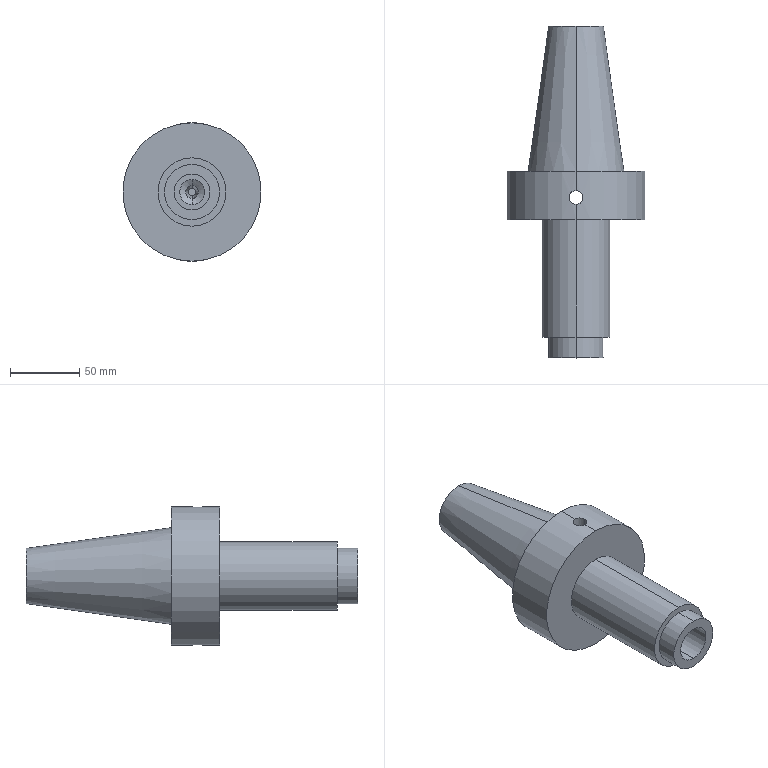Part | SolidWorks | features ICE 2, 3DProfileFeature 1, HoleWzd 1, RevolutionThin 1 | 1 solid | 31 faces | box 100 x 240 x 100 mm | volume 634336 mm3 | cylinder 16 | plane 9 | cone 6 | commonest cylinder face diameters 9.4 x4 10 x2 18 x2 26 x2 40 x2 49.4 x2
STEP:
#1=CARTESIAN_POINT('',(0.,220.,2.654));
#2=VERTEX_POINT('',#1);
#3=CARTESIAN_POINT('',(0.,220.,-2.654));
#4=VERTEX_POINT('',#3);
#5=CARTESIAN_POINT('',(0.,220.,0.));
#6=DIRECTION('',(0.,-1.,0.));
#7=DIRECTION('',(0.,0.,-1.));
#8=AXIS2_PLACEMENT_3D('',#5,#6,#7);
#9=CIRCLE('',#8,2.654);
#10=EDGE_CURVE('',#2,#4,#9,.T.);
#11=ORIENTED_EDGE('',*,*,#10,.F.);
#12=CARTESIAN_POINT('',(0.,121.,16.797));
#13=VERTEX_POINT('',#12);
#14=CARTESIAN_POINT('',(0.,220.,2.654));
#15=DIRECTION('',(0.,-0.9899,0.1414));
#16=VECTOR('',#15,1000.);
#17=LINE('',#14,#16);
#18=EDGE_CURVE('',#2,#13,#17,.T.);
#19=ORIENTED_EDGE('',*,*,#18,.T.);
#20=CARTESIAN_POINT('',(-3.,120.,16.672));
#21=VERTEX_POINT('',#20);
#22=CARTESIAN_POINT('',(-3.,120.,16.672));
#23=CARTESIAN_POINT('',(-2.567,120.325,16.703));
#24=CARTESIAN_POINT('',(-2.094,120.572,16.735));
#25=CARTESIAN_POINT('',(-1.326,120.829,16.771));
#26=CARTESIAN_POINT('',(-1.064,120.893,16.781));
#27=CARTESIAN_POINT('',(-0.5365,120.978,16.794));
#28=CARTESIAN_POINT('',(-0.2698,121.,16.797));
#29=CARTESIAN_POINT('',(0.,121.,16.797));
#30=B_SPLINE_CURVE_WITH_KNOTS('',3,(#22,#23,#24,#25,#26,#27,#28,#29),.UNSPECIFIED.,.F.,.F.,(4,2,2,4),(0.000000329,0.001604,0.002405,0.003207),.UNSPECIFIED.);
#31=EDGE_CURVE('',#21,#13,#30,.T.);
#32=ORIENTED_EDGE('',*,*,#31,.F.);
#33=CARTESIAN_POINT('',(-3.,120.,-16.672));
#34=VERTEX_POINT('',#33);
#35=CARTESIAN_POINT('',(0.,120.,0.));
#36=DIRECTION('',(0.,-1.,0.));
#37=DIRECTION('',(0.,0.,-1.));
#38=AXIS2_PLACEMENT_3D('',#35,#36,#37);
#39=CIRCLE('',#38,16.94);
#40=EDGE_CURVE('',#21,#34,#39,.T.);
#41=ORIENTED_EDGE('',*,*,#40,.T.);
#42=CARTESIAN_POINT('',(0.,121.,-16.797));
#43=VERTEX_POINT('',#42);
#44=CARTESIAN_POINT('',(0.,121.,-16.797));
#45=CARTESIAN_POINT('',(-0.2692,121.,-16.797));
#46=CARTESIAN_POINT('',(-0.5388,120.978,-16.794));
#47=CARTESIAN_POINT('',(-1.065,120.892,-16.781));
#48=CARTESIAN_POINT('',(-1.325,120.829,-16.771));
#49=CARTESIAN_POINT('',(-1.834,120.659,-16.747));
#50=CARTESIAN_POINT('',(-2.083,120.553,-16.733));
#51=CARTESIAN_POINT('',(-2.557,120.305,-16.703));
#52=CARTESIAN_POINT('',(-2.784,120.162,-16.687));
#53=CARTESIAN_POINT('',(-3.,120.,-16.672));
#54=B_SPLINE_CURVE_WITH_KNOTS('',3,(#44,#45,#46,#47,#48,#49,#50,#51,#52,#53),.UNSPECIFIED.,.F.,.F.,(4,2,2,2,4),(0.003207,0.004007,0.004807,0.005607,0.006407),.UNSPECIFIED.);
#55=EDGE_CURVE('',#43,#34,#54,.T.);
#56=ORIENTED_EDGE('',*,*,#55,.F.);
#57=CARTESIAN_POINT('',(0.,220.,-2.654));
#58=DIRECTION('',(0.,-0.9899,-0.1414));
#59=VECTOR('',#58,1000.);
#60=LINE('',#57,#59);
#61=EDGE_CURVE('',#4,#43,#60,.T.);
#62=ORIENTED_EDGE('',*,*,#61,.F.);
#63=EDGE_LOOP('',(#11,#19,#32,#41,#56,#62));
#64=FACE_OUTER_BOUND('',#63,.T.);
#65=CARTESIAN_POINT('',(0.,220.,0.));
#66=DIRECTION('',(0.,-1.,0.));
#67=DIRECTION('',(0.,0.,-1.));
#68=AXIS2_PLACEMENT_3D('',#65,#66,#67);
#69=CONICAL_SURFACE('',#68,2.654,0.1419);
#70=ADVANCED_FACE('',(#64),#69,.F.);
#71=CARTESIAN_POINT('',(0.,111.,-4.7));
#72=VERTEX_POINT('',#71);
#73=CARTESIAN_POINT('',(0.,111.,4.7));
#74=VERTEX_POINT('',#73);
#75=CARTESIAN_POINT('',(0.,111.,-4.7));
#76=CARTESIAN_POINT('',(0.3471,111.,-4.7));
#77=CARTESIAN_POINT('',(0.6844,111.036,-4.662));
#78=CARTESIAN_POINT('',(1.177,111.138,-4.553));
#79=CARTESIAN_POINT('',(1.34,111.18,-4.508));
#80=CARTESIAN_POINT('',(1.652,111.278,-4.403));
#81=CARTESIAN_POINT('',(1.803,111.334,-4.343));
#82=CARTESIAN_POINT('',(2.239,111.518,-4.145));
#83=CARTESIAN_POINT('',(2.511,111.667,-3.984));
#84=CARTESIAN_POINT('',(3.,111.989,-3.631));
#85=CARTESIAN_POINT('',(3.219,112.164,-3.437));
#86=CARTESIAN_POINT('',(3.615,112.535,-3.017));
#87=CARTESIAN_POINT('',(3.791,112.73,-2.792));
#88=CARTESIAN_POINT('',(4.095,113.12,-2.323));
#89=CARTESIAN_POINT('',(4.225,113.317,-2.078));
#90=CARTESIAN_POINT('',(4.444,113.699,-1.555));
#91=CARTESIAN_POINT('',(4.534,113.886,-1.276));
#92=CARTESIAN_POINT('',(4.63,114.111,-0.8215));
#93=CARTESIAN_POINT('',(4.656,114.177,-0.6619));
#94=CARTESIAN_POINT('',(4.691,114.269,-0.3332));
#95=CARTESIAN_POINT('',(4.7,114.295,-0.1601));
#96=CARTESIAN_POINT('',(4.7,114.293,0.1835));
#97=CARTESIAN_POINT('',(4.69,114.265,0.3527));
#98=CARTESIAN_POINT('',(4.653,114.169,0.6836));
#99=CARTESIAN_POINT('',(4.627,114.103,0.8395));
#100=CARTESIAN_POINT('',(4.562,113.952,1.14));
#101=CARTESIAN_POINT('',(4.523,113.867,1.285));
#102=CARTESIAN_POINT('',(4.434,113.688,1.565));
#103=CARTESIAN_POINT('',(4.385,113.594,1.699));
#104=CARTESIAN_POINT('',(4.22,113.309,2.089));
#105=CARTESIAN_POINT('',(4.089,113.112,2.335));
#106=CARTESIAN_POINT('',(3.782,112.719,2.805));
#107=CARTESIAN_POINT('',(3.605,112.525,3.029));
#108=CARTESIAN_POINT('',(3.212,112.159,3.443));
#109=CARTESIAN_POINT('',(2.994,111.985,3.635));
#110=CARTESIAN_POINT('',(2.506,111.663,3.988));
#111=CARTESIAN_POINT('',(2.234,111.516,4.147));
#112=CARTESIAN_POINT('',(1.799,111.332,4.345));
#113=CARTESIAN_POINT('',(1.648,111.277,4.405));
#114=CARTESIAN_POINT('',(1.336,111.179,4.509));
#115=CARTESIAN_POINT('',(1.173,111.137,4.554));
#116=CARTESIAN_POINT('',(0.6824,111.036,4.662));
#117=CARTESIAN_POINT('',(0.3462,111.,4.7));
#118=CARTESIAN_POINT('',(0.,111.,4.7));
#119=B_SPLINE_CURVE_WITH_KNOTS('',3,(#75,#76,#77,#78,#79,#80,#81,#82,#83,#84,#85,#86,#87,#88,#89,#90,#91,#92,#93,#94,#95,#96,#97,#98,#99,#100,#101,#102,#103,#104,#105,#106,#107,#108,#109,#110,#111,#112,#113,#114,#115,#116,#117,#118),.UNSPECIFIED.,.F.,.F.,(4,2,2,2,2,2,2,2,2,2,2,2,2,2,2,2,2,2,2,2,2,4),(0.,0.001023,0.001535,0.002047,0.00307,0.004094,0.005117,0.00614,0.007164,0.007675,0.008187,0.008699,0.009211,0.009722,0.01023,0.01126,0.01228,0.0133,0.01433,0.01484,0.01535,0.01637),.UNSPECIFIED.);
#120=EDGE_CURVE('',#72,#74,#119,.T.);
#121=ORIENTED_EDGE('',*,*,#120,.T.);
#122=CARTESIAN_POINT('',(0.,111.,4.7));
#123=CARTESIAN_POINT('',(-0.3464,111.,4.7));
#124=CARTESIAN_POINT('',(-0.6849,111.036,4.662));
#125=CARTESIAN_POINT('',(-1.179,111.138,4.553));
#126=CARTESIAN_POINT('',(-1.341,111.18,4.508));
#127=CARTESIAN_POINT('',(-1.653,111.278,4.403));
#128=CARTESIAN_POINT('',(-1.804,111.334,4.343));
#129=CARTESIAN_POINT('',(-2.095,111.457,4.21));
#130=CARTESIAN_POINT('',(-2.237,111.526,4.136));
#131=CARTESIAN_POINT('',(-2.506,111.671,3.979));
#132=CARTESIAN_POINT('',(-2.634,111.748,3.895));
#133=CARTESIAN_POINT('',(-3.,111.989,3.631));
#134=CARTESIAN_POINT('',(-3.219,112.165,3.437));
#135=CARTESIAN_POINT('',(-3.617,112.537,3.015));
#136=CARTESIAN_POINT('',(-3.791,112.731,2.792));
#137=CARTESIAN_POINT('',(-4.095,113.12,2.324));
#138=CARTESIAN_POINT('',(-4.225,113.317,2.079));
#139=CARTESIAN_POINT('',(-4.445,113.699,1.554));
#140=CARTESIAN_POINT('',(-4.534,113.886,1.276));
#141=CARTESIAN_POINT('',(-4.63,114.111,0.8211));
#142=CARTESIAN_POINT('',(-4.656,114.177,0.6623));
#143=CARTESIAN_POINT('',(-4.691,114.269,0.3341));
#144=CARTESIAN_POINT('',(-4.7,114.295,0.1602));
#145=CARTESIAN_POINT('',(-4.7,114.293,-0.1811));
#146=CARTESIAN_POINT('',(-4.69,114.265,-0.3517));
#147=CARTESIAN_POINT('',(-4.653,114.17,-0.681));
#148=CARTESIAN_POINT('',(-4.627,114.104,-0.8368));
#149=CARTESIAN_POINT('',(-4.563,113.954,-1.138));
#150=CARTESIAN_POINT('',(-4.524,113.868,-1.283));
#151=CARTESIAN_POINT('',(-4.435,113.69,-1.562));
#152=CARTESIAN_POINT('',(-4.386,113.597,-1.695));
#153=CARTESIAN_POINT('',(-4.221,113.311,-2.086));
#154=CARTESIAN_POINT('',(-4.09,113.114,-2.332));
#155=CARTESIAN_POINT('',(-3.783,112.721,-2.804));
#156=CARTESIAN_POINT('',(-3.609,112.529,-3.025));
#157=CARTESIAN_POINT('',(-3.216,112.162,-3.439));
#158=CARTESIAN_POINT('',(-2.997,111.987,-3.633));
#159=CARTESIAN_POINT('',(-2.505,111.662,-3.989));
#160=CARTESIAN_POINT('',(-2.238,111.518,-4.145));
#161=CARTESIAN_POINT('',(-1.658,111.272,-4.409));
#162=CARTESIAN_POINT('',(-1.342,111.172,-4.517));
#163=CARTESIAN_POINT('',(-0.6898,111.037,-4.661));
#164=CARTESIAN_POINT('',(-0.3472,111.,-4.7));
#165=CARTESIAN_POINT('',(0.,111.,-4.7));
#166=B_SPLINE_CURVE_WITH_KNOTS('',3,(#122,#123,#124,#125,#126,#127,#128,#129,#130,#131,#132,#133,#134,#135,#136,#137,#138,#139,#140,#141,#142,#143,#144,#145,#146,#147,#148,#149,#150,#151,#152,#153,#154,#155,#156,#157,#158,#159,#160,#161,#162,#163,#164,#165),.UNSPECIFIED.,.F.,.F.,(4,2,2,2,2,2,2,2,2,2,2,2,2,2,2,2,2,2,2,2,2,4),(0.01637,0.0174,0.01791,0.01842,0.01893,0.01945,0.02047,0.02149,0.02252,0.02354,0.02405,0.02456,0.02508,0.02559,0.0261,0.02661,0.02764,0.02866,0.02968,0.03071,0.03173,0.03276),.UNSPECIFIED.);
#167=EDGE_CURVE('',#74,#72,#166,.T.);
#168=ORIENTED_EDGE('',*,*,#167,.T.);
#169=EDGE_LOOP('',(#121,#168));
#170=FACE_BOUND('',#169,.T.);
#171=CARTESIAN_POINT('',(-5.,116.,-49.749));
#172=VERTEX_POINT('',#171);
#173=CARTESIAN_POINT('',(0.,111.,-50.));
#174=VERTEX_POINT('',#173);
#175=CARTESIAN_POINT('',(-5.,116.,-49.749));
#176=CARTESIAN_POINT('',(-5.,115.674,-49.749));
#177=CARTESIAN_POINT('',(-4.967,115.342,-49.753));
#178=CARTESIAN_POINT('',(-4.839,114.701,-49.765));
#179=CARTESIAN_POINT('',(-4.745,114.389,-49.775));
#180=CARTESIAN_POINT('',(-4.557,113.935,-49.792));
#181=CARTESIAN_POINT('',(-4.486,113.785,-49.798));
#182=CARTESIAN_POINT('',(-4.331,113.496,-49.812));
#183=CARTESIAN_POINT('',(-4.247,113.356,-49.819));
#184=CARTESIAN_POINT('',(-3.975,112.95,-49.842));
#185=CARTESIAN_POINT('',(-3.769,112.698,-49.858));
#186=CARTESIAN_POINT('',(-3.302,112.231,-49.891));
#187=CARTESIAN_POINT('',(-3.05,112.024,-49.908));
#188=CARTESIAN_POINT('',(-2.644,111.753,-49.93));
#189=CARTESIAN_POINT('',(-2.504,111.669,-49.937));
#190=CARTESIAN_POINT('',(-2.214,111.514,-49.951));
#191=CARTESIAN_POINT('',(-2.065,111.443,-49.958));
#192=CARTESIAN_POINT('',(-1.61,111.255,-49.975));
#193=CARTESIAN_POINT('',(-1.299,111.161,-49.984));
#194=CARTESIAN_POINT('',(-0.6578,111.033,-49.997));
#195=CARTESIAN_POINT('',(-0.3264,111.,-50.));
#196=CARTESIAN_POINT('',(0.,111.,-50.));
#197=B_SPLINE_CURVE_WITH_KNOTS('',3,(#175,#176,#177,#178,#179,#180,#181,#182,#183,#184,#185,#186,#187,#188,#189,#190,#191,#192,#193,#194,#195,#196),.UNSPECIFIED.,.F.,.F.,(4,2,2,2,2,2,2,2,2,2,4),(0.007823,0.0088,0.009778,0.01027,0.01076,0.01173,0.01271,0.0132,0.01369,0.01466,0.01564),.UNSPECIFIED.);
#198=EDGE_CURVE('',#172,#174,#197,.T.);
#199=ORIENTED_EDGE('',*,*,#198,.F.);
#200=CARTESIAN_POINT('',(-5.,116.,49.749));
#201=VERTEX_POINT('',#200);
#202=CARTESIAN_POINT('',(-5.,116.,-50.));
#203=DIRECTION('',(0.,0.,1.));
#204=VECTOR('',#203,1000.);
#205=LINE('',#202,#204);
#206=EDGE_CURVE('',#172,#201,#205,.T.);
#207=ORIENTED_EDGE('',*,*,#206,.T.);
#208=CARTESIAN_POINT('',(0.,111.,50.));
#209=VERTEX_POINT('',#208);
#210=CARTESIAN_POINT('',(0.,111.,50.));
#211=CARTESIAN_POINT('',(-0.3263,111.,50.));
#212=CARTESIAN_POINT('',(-0.6577,111.033,49.997));
#213=CARTESIAN_POINT('',(-1.299,111.161,49.984));
#214=CARTESIAN_POINT('',(-1.611,111.255,49.975));
#215=CARTESIAN_POINT('',(-2.065,111.443,49.958));
#216=CARTESIAN_POINT('',(-2.215,111.514,49.951));
#217=CARTESIAN_POINT('',(-2.504,111.669,49.937));
#218=CARTESIAN_POINT('',(-2.644,111.753,49.93));
#219=CARTESIAN_POINT('',(-3.05,112.025,49.908));
#220=CARTESIAN_POINT('',(-3.302,112.231,49.891));
#221=CARTESIAN_POINT('',(-3.769,112.698,49.858));
#222=CARTESIAN_POINT('',(-3.976,112.95,49.842));
#223=CARTESIAN_POINT('',(-4.247,113.356,49.819));
#224=CARTESIAN_POINT('',(-4.331,113.496,49.812));
#225=CARTESIAN_POINT('',(-4.486,113.786,49.798));
#226=CARTESIAN_POINT('',(-4.557,113.935,49.792));
#227=CARTESIAN_POINT('',(-4.745,114.39,49.775));
#228=CARTESIAN_POINT('',(-4.839,114.701,49.765));
#229=CARTESIAN_POINT('',(-4.967,115.342,49.753));
#230=CARTESIAN_POINT('',(-5.,115.674,49.749));
#231=CARTESIAN_POINT('',(-5.,116.,49.749));
#232=B_SPLINE_CURVE_WITH_KNOTS('',3,(#210,#211,#212,#213,#214,#215,#216,#217,#218,#219,#220,#221,#222,#223,#224,#225,#226,#227,#228,#229,#230,#231),.UNSPECIFIED.,.F.,.F.,(4,2,2,2,2,2,2,2,2,2,4),(0.007823,0.0088,0.009778,0.01027,0.01076,0.01173,0.01271,0.0132,0.01369,0.01466,0.01564),.UNSPECIFIED.);
#233=EDGE_CURVE('',#209,#201,#232,.T.);
#234=ORIENTED_EDGE('',*,*,#233,.F.);
#235=CARTESIAN_POINT('',(5.,116.,49.749));
#236=VERTEX_POINT('',#235);
#237=CARTESIAN_POINT('',(5.,116.,49.749));
#238=CARTESIAN_POINT('',(5.,115.669,49.749));
#239=CARTESIAN_POINT('',(4.968,115.344,49.753));
#240=CARTESIAN_POINT('',(4.872,114.865,49.762));
#241=CARTESIAN_POINT('',(4.832,114.706,49.766));
#242=CARTESIAN_POINT('',(4.737,114.392,49.775));
#243=CARTESIAN_POINT('',(4.681,114.236,49.78));
#244=CARTESIAN_POINT('',(4.493,113.781,49.798));
#245=CARTESIAN_POINT('',(4.339,113.494,49.812));
#246=CARTESIAN_POINT('',(3.976,112.951,49.842));
#247=CARTESIAN_POINT('',(3.765,112.694,49.859));
#248=CARTESIAN_POINT('',(3.304,112.233,49.891));
#249=CARTESIAN_POINT('',(3.052,112.026,49.908));
#250=CARTESIAN_POINT('',(2.505,111.66,49.938));
#251=CARTESIAN_POINT('',(2.214,111.505,49.952));
#252=CARTESIAN_POINT('',(1.612,111.256,49.975));
#253=CARTESIAN_POINT('',(1.297,111.16,49.984));
#254=CARTESIAN_POINT('',(0.6511,111.032,49.997));
#255=CARTESIAN_POINT('',(0.3264,111.,50.));
#256=CARTESIAN_POINT('',(0.,111.,50.));
#257=B_SPLINE_CURVE_WITH_KNOTS('',3,(#237,#238,#239,#240,#241,#242,#243,#244,#245,#246,#247,#248,#249,#250,#251,#252,#253,#254,#255,#256),.UNSPECIFIED.,.F.,.F.,(4,2,2,2,2,2,2,2,2,4),(0.,0.0009779,0.001467,0.001956,0.002934,0.003911,0.004889,0.005867,0.006845,0.007823),.UNSPECIFIED.);
#258=EDGE_CURVE('',#236,#209,#257,.T.);
#259=ORIENTED_EDGE('',*,*,#258,.F.);
#260=CARTESIAN_POINT('',(5.,116.,-49.749));
#261=VERTEX_POINT('',#260);
#262=CARTESIAN_POINT('',(5.,116.,-50.));
#263=DIRECTION('',(0.,0.,1.));
#264=VECTOR('',#263,1000.);
#265=LINE('',#262,#264);
#266=EDGE_CURVE('',#261,#236,#265,.T.);
#267=ORIENTED_EDGE('',*,*,#266,.F.);
#268=CARTESIAN_POINT('',(0.,111.,-50.));
#269=CARTESIAN_POINT('',(0.3265,111.,-50.));
#270=CARTESIAN_POINT('',(0.6512,111.032,-49.997));
#271=CARTESIAN_POINT('',(1.297,111.16,-49.984));
#272=CARTESIAN_POINT('',(1.612,111.256,-49.975));
#273=CARTESIAN_POINT('',(2.214,111.505,-49.952));
#274=CARTESIAN_POINT('',(2.505,111.66,-49.938));
#275=CARTESIAN_POINT('',(3.052,112.026,-49.908));
#276=CARTESIAN_POINT('',(3.304,112.233,-49.891));
#277=CARTESIAN_POINT('',(3.765,112.694,-49.859));
#278=CARTESIAN_POINT('',(3.976,112.951,-49.842));
#279=CARTESIAN_POINT('',(4.339,113.495,-49.812));
#280=CARTESIAN_POINT('',(4.493,113.782,-49.798));
#281=CARTESIAN_POINT('',(4.681,114.236,-49.78));
#282=CARTESIAN_POINT('',(4.737,114.392,-49.775));
#283=CARTESIAN_POINT('',(4.833,114.706,-49.766));
#284=CARTESIAN_POINT('',(4.872,114.865,-49.762));
#285=CARTESIAN_POINT('',(4.968,115.344,-49.753));
#286=CARTESIAN_POINT('',(5.,115.669,-49.749));
#287=CARTESIAN_POINT('',(5.,116.,-49.749));
#288=B_SPLINE_CURVE_WITH_KNOTS('',3,(#268,#269,#270,#271,#272,#273,#274,#275,#276,#277,#278,#279,#280,#281,#282,#283,#284,#285,#286,#287),.UNSPECIFIED.,.F.,.F.,(4,2,2,2,2,2,2,2,2,4),(0.01564,0.01662,0.0176,0.01858,0.01955,0.02053,0.02151,0.022,0.02249,0.02347),.UNSPECIFIED.);
#289=EDGE_CURVE('',#174,#261,#288,.T.);
#290=ORIENTED_EDGE('',*,*,#289,.F.);
#291=EDGE_LOOP('',(#199,#207,#234,#259,#267,#290));
#292=FACE_OUTER_BOUND('',#291,.T.);
#293=CARTESIAN_POINT('',(0.,116.,-50.));
#294=DIRECTION('',(0.,0.,1.));
#295=DIRECTION('',(1.,0.,0.));
#296=AXIS2_PLACEMENT_3D('',#293,#294,#295);
#297=CYLINDRICAL_SURFACE('',#296,5.);
#298=ADVANCED_FACE('',(#170,#292),#297,.F.);
#299=ORIENTED_EDGE('',*,*,#167,.F.);
#300=CARTESIAN_POINT('',(0.,87.583,4.7));
#301=VERTEX_POINT('',#300);
#302=CARTESIAN_POINT('',(0.,0.,4.7));
#303=DIRECTION('',(0.,-1.,0.));
#304=VECTOR('',#303,1000.);
#305=LINE('',#302,#304);
#306=EDGE_CURVE('',#74,#301,#305,.T.);
#307=ORIENTED_EDGE('',*,*,#306,.T.);
#308=CARTESIAN_POINT('',(0.,87.583,-4.7));
#309=VERTEX_POINT('',#308);
#310=CARTESIAN_POINT('',(0.,87.583,-4.7));
#311=CARTESIAN_POINT('',(-0.3072,87.578,-4.7));
#312=CARTESIAN_POINT('',(-0.6118,87.573,-4.67));
#313=CARTESIAN_POINT('',(-1.216,87.563,-4.55));
#314=CARTESIAN_POINT('',(-1.514,87.558,-4.46));
#315=CARTESIAN_POINT('',(-2.08,87.549,-4.226));
#316=CARTESIAN_POINT('',(-2.351,87.545,-4.082));
#317=CARTESIAN_POINT('',(-2.867,87.537,-3.737));
#318=CARTESIAN_POINT('',(-3.105,87.533,-3.542));
#319=CARTESIAN_POINT('',(-3.541,87.526,-3.106));
#320=CARTESIAN_POINT('',(-3.739,87.523,-2.865));
#321=CARTESIAN_POINT('',(-4.08,87.518,-2.353));
#322=CARTESIAN_POINT('',(-4.227,87.515,-2.079));
#323=CARTESIAN_POINT('',(-4.462,87.512,-1.508));
#324=CARTESIAN_POINT('',(-4.551,87.51,-1.215));
#325=CARTESIAN_POINT('',(-4.67,87.509,-0.6132));
#326=CARTESIAN_POINT('',(-4.7,87.508,-0.3017));
#327=CARTESIAN_POINT('',(-4.7,87.508,0.3122));
#328=CARTESIAN_POINT('',(-4.67,87.509,0.6168));
#329=CARTESIAN_POINT('',(-4.549,87.51,1.221));
#330=CARTESIAN_POINT('',(-4.458,87.512,1.519));
#331=CARTESIAN_POINT('',(-4.223,87.516,2.085));
#332=CARTESIAN_POINT('',(-4.079,87.518,2.356));
#333=CARTESIAN_POINT('',(-3.734,87.523,2.872));
#334=CARTESIAN_POINT('',(-3.539,87.526,3.108));
#335=CARTESIAN_POINT('',(-3.106,87.533,3.541));
#336=CARTESIAN_POINT('',(-2.864,87.537,3.739));
#337=CARTESIAN_POINT('',(-2.352,87.545,4.081));
#338=CARTESIAN_POINT('',(-2.082,87.549,4.225));
#339=CARTESIAN_POINT('',(-1.514,87.558,4.46));
#340=CARTESIAN_POINT('',(-1.215,87.563,4.551));
#341=CARTESIAN_POINT('',(-0.6141,87.573,4.67));
#342=CARTESIAN_POINT('',(-0.3092,87.578,4.7));
#343=CARTESIAN_POINT('',(0.,87.583,4.7));
#344=B_SPLINE_CURVE_WITH_KNOTS('',3,(#310,#311,#312,#313,#314,#315,#316,#317,#318,#319,#320,#321,#322,#323,#324,#325,#326,#327,#328,#329,#330,#331,#332,#333,#334,#335,#336,#337,#338,#339,#340,#341,#342,#343),.UNSPECIFIED.,.F.,.F.,(4,2,2,2,2,2,2,2,2,2,2,2,2,2,2,2,4),(0.02547,0.02639,0.02731,0.02823,0.02916,0.03008,0.031,0.03192,0.03285,0.03377,0.03469,0.03561,0.03653,0.03746,0.03838,0.0393,0.04022),.UNSPECIFIED.);
#345=EDGE_CURVE('',#309,#301,#344,.T.);
#346=ORIENTED_EDGE('',*,*,#345,.F.);
#347=CARTESIAN_POINT('',(0.,0.,-4.7));
#348=DIRECTION('',(0.,-1.,0.));
#349=VECTOR('',#348,1000.);
#350=LINE('',#347,#349);
#351=EDGE_CURVE('',#72,#309,#350,.T.);
#352=ORIENTED_EDGE('',*,*,#351,.F.);
#353=EDGE_LOOP('',(#299,#307,#346,#352));
#354=FACE_OUTER_BOUND('',#353,.T.);
#355=CARTESIAN_POINT('',(0.,0.,0.));
#356=DIRECTION('',(0.,-1.,0.));
#357=DIRECTION('',(0.,0.,-1.));
#358=AXIS2_PLACEMENT_3D('',#355,#356,#357);
#359=CYLINDRICAL_SURFACE('',#358,4.7);
#360=ADVANCED_FACE('',(#354),#359,.F.);
#361=CARTESIAN_POINT('',(0.1259,85.,9.));
#362=VERTEX_POINT('',#361);
#363=CARTESIAN_POINT('',(0.1259,85.,-9.));
#364=VERTEX_POINT('',#363);
#365=CARTESIAN_POINT('',(0.1259,85.,0.));
#366=DIRECTION('',(0.,-1.,0.));
#367=DIRECTION('',(0.,0.,-1.));
#368=AXIS2_PLACEMENT_3D('',#365,#366,#367);
#369=CIRCLE('',#368,9.);
#370=EDGE_CURVE('',#362,#364,#369,.T.);
#371=ORIENTED_EDGE('',*,*,#370,.F.);
#372=CARTESIAN_POINT('',(0.1259,40.,9.));
#373=VERTEX_POINT('',#372);
#374=CARTESIAN_POINT('',(0.1259,40.,9.));
#375=DIRECTION('',(0.,-1.,0.));
#376=VECTOR('',#375,1000.);
#377=LINE('',#374,#376);
#378=EDGE_CURVE('',#362,#373,#377,.T.);
#379=ORIENTED_EDGE('',*,*,#378,.T.);
#380=CARTESIAN_POINT('',(0.1259,40.,-9.));
#381=VERTEX_POINT('',#380);
#382=CARTESIAN_POINT('',(0.1259,40.,0.));
#383=DIRECTION('',(0.,-1.,0.));
#384=DIRECTION('',(0.,0.,-1.));
#385=AXIS2_PLACEMENT_3D('',#382,#383,#384);
#386=CIRCLE('',#385,9.);
#387=EDGE_CURVE('',#373,#381,#386,.T.);
#388=ORIENTED_EDGE('',*,*,#387,.T.);
#389=CARTESIAN_POINT('',(0.1259,40.,-9.));
#390=DIRECTION('',(0.,-1.,0.));
#391=VECTOR('',#390,1000.);
#392=LINE('',#389,#391);
#393=EDGE_CURVE('',#364,#381,#392,.T.);
#394=ORIENTED_EDGE('',*,*,#393,.F.);
#395=EDGE_LOOP('',(#371,#379,#388,#394));
#396=FACE_OUTER_BOUND('',#395,.T.);
#397=CARTESIAN_POINT('',(0.1259,40.,0.));
#398=DIRECTION('',(0.,-1.,0.));
#399=DIRECTION('',(0.,0.,-1.));
#400=AXIS2_PLACEMENT_3D('',#397,#398,#399);
#401=CYLINDRICAL_SURFACE('',#400,9.);
#402=ADVANCED_FACE('',(#396),#401,.F.);
#403=CARTESIAN_POINT('',(0.1259,87.585,-4.698));
#404=VERTEX_POINT('',#403);
#405=CARTESIAN_POINT('',(0.1259,87.585,-4.698));
#406=CARTESIAN_POINT('',(0.1049,87.584,-4.699));
#407=CARTESIAN_POINT('',(0.06291,87.584,-4.7));
#408=CARTESIAN_POINT('',(0.02096,87.583,-4.7));
#409=CARTESIAN_POINT('',(0.,87.583,-4.7));
#410=B_SPLINE_CURVE_WITH_KNOTS('',3,(#405,#406,#407,#408,#409),.UNSPECIFIED.,.F.,.F.,(4,1,4),(0.02534,0.0254,0.02547),.UNSPECIFIED.);
#411=EDGE_CURVE('',#404,#309,#410,.T.);
#412=ORIENTED_EDGE('',*,*,#411,.T.);
#413=ORIENTED_EDGE('',*,*,#345,.T.);
#414=CARTESIAN_POINT('',(0.1259,87.585,4.698));
#415=VERTEX_POINT('',#414);
#416=CARTESIAN_POINT('',(0.,87.583,4.7));
#417=CARTESIAN_POINT('',(0.02095,87.583,4.7));
#418=CARTESIAN_POINT('',(0.04191,87.583,4.7));
#419=CARTESIAN_POINT('',(0.08389,87.584,4.699));
#420=CARTESIAN_POINT('',(0.1049,87.584,4.699));
#421=CARTESIAN_POINT('',(0.1259,87.585,4.698));
#422=B_SPLINE_CURVE_WITH_KNOTS('',3,(#416,#417,#418,#419,#420,#421),.UNSPECIFIED.,.F.,.F.,(4,2,4),(0.0107,0.01077,0.01083),.UNSPECIFIED.);
#423=EDGE_CURVE('',#301,#415,#422,.T.);
#424=ORIENTED_EDGE('',*,*,#423,.T.);
#425=CARTESIAN_POINT('',(0.1259,85.,9.));
#426=DIRECTION('',(0.,-0.515,0.8572));
#427=VECTOR('',#426,1000.);
#428=LINE('',#425,#427);
#429=EDGE_CURVE('',#415,#362,#428,.T.);
#430=ORIENTED_EDGE('',*,*,#429,.T.);
#431=ORIENTED_EDGE('',*,*,#370,.T.);
#432=CARTESIAN_POINT('',(0.1259,85.,-9.));
#433=DIRECTION('',(0.,-0.515,-0.8572));
#434=VECTOR('',#433,1000.);
#435=LINE('',#432,#434);
#436=EDGE_CURVE('',#404,#364,#435,.T.);
#437=ORIENTED_EDGE('',*,*,#436,.F.);
#438=EDGE_LOOP('',(#412,#413,#424,#430,#431,#437));
#439=FACE_OUTER_BOUND('',#438,.T.);
#440=CARTESIAN_POINT('',(0.1259,85.,0.));
#441=DIRECTION('',(0.,-1.,0.));
#442=DIRECTION('',(0.,0.,-1.));
#443=AXIS2_PLACEMENT_3D('',#440,#441,#442);
#444=CONICAL_SURFACE('',#443,9.,1.03);
#445=ADVANCED_FACE('',(#439),#444,.F.);
#446=CARTESIAN_POINT('',(0.,240.,-20.));
#447=VERTEX_POINT('',#446);
#448=CARTESIAN_POINT('',(0.,240.,20.));
#449=VERTEX_POINT('',#448);
#450=CARTESIAN_POINT('',(0.,240.,0.));
#451=DIRECTION('',(0.,-1.,0.));
#452=DIRECTION('',(0.,0.,-1.));
#453=AXIS2_PLACEMENT_3D('',#450,#451,#452);
#454=CIRCLE('',#453,20.);
#455=EDGE_CURVE('',#447,#449,#454,.T.);
#456=ORIENTED_EDGE('',*,*,#455,.T.);
#457=CARTESIAN_POINT('',(0.,135.,35.));
#458=VERTEX_POINT('',#457);
#459=CARTESIAN_POINT('',(0.,240.,20.));
#460=DIRECTION('',(0.,-0.9899,0.1414));
#461=VECTOR('',#460,1000.);
#462=LINE('',#459,#461);
#463=EDGE_CURVE('',#449,#458,#462,.T.);
#464=ORIENTED_EDGE('',*,*,#463,.T.);
#465=CARTESIAN_POINT('',(0.,135.,-35.));
#466=VERTEX_POINT('',#465);
#467=CARTESIAN_POINT('',(0.,135.,0.));
#468=DIRECTION('',(0.,-1.,0.));
#469=DIRECTION('',(0.,0.,-1.));
#470=AXIS2_PLACEMENT_3D('',#467,#468,#469);
#471=CIRCLE('',#470,35.);
#472=EDGE_CURVE('',#466,#458,#471,.T.);
#473=ORIENTED_EDGE('',*,*,#472,.F.);
#474=CARTESIAN_POINT('',(0.,240.,-20.));
#475=DIRECTION('',(0.,-0.9899,-0.1414));
#476=VECTOR('',#475,1000.);
#477=LINE('',#474,#476);
#478=EDGE_CURVE('',#447,#466,#477,.T.);
#479=ORIENTED_EDGE('',*,*,#478,.F.);
#480=EDGE_LOOP('',(#456,#464,#473,#479));
#481=FACE_OUTER_BOUND('',#480,.T.);
#482=CARTESIAN_POINT('',(0.,240.,0.));
#483=DIRECTION('',(0.,-1.,0.));
#484=DIRECTION('',(0.,0.,-1.));
#485=AXIS2_PLACEMENT_3D('',#482,#483,#484);
#486=CONICAL_SURFACE('',#485,20.,0.1419);
#487=ADVANCED_FACE('',(#481),#486,.T.);
#488=CARTESIAN_POINT('',(0.,135.,-50.));
#489=VERTEX_POINT('',#488);
#490=CARTESIAN_POINT('',(0.,135.,50.));
#491=VERTEX_POINT('',#490);
#492=CARTESIAN_POINT('',(0.,135.,0.));
#493=DIRECTION('',(0.,-1.,0.));
#494=DIRECTION('',(0.,0.,-1.));
#495=AXIS2_PLACEMENT_3D('',#492,#493,#494);
#496=CIRCLE('',#495,50.);
#497=EDGE_CURVE('',#489,#491,#496,.T.);
#498=ORIENTED_EDGE('',*,*,#497,.T.);
#499=CARTESIAN_POINT('',(0.,121.,50.));
#500=VERTEX_POINT('',#499);
#501=CARTESIAN_POINT('',(0.,0.,50.));
#502=DIRECTION('',(0.,-1.,0.));
#503=VECTOR('',#502,1000.);
#504=LINE('',#501,#503);
#505=EDGE_CURVE('',#491,#500,#504,.T.);
#506=ORIENTED_EDGE('',*,*,#505,.T.);
#507=CARTESIAN_POINT('',(0.,121.,50.));
#508=CARTESIAN_POINT('',(0.3302,121.,50.));
#509=CARTESIAN_POINT('',(0.6554,120.968,49.997));
#510=CARTESIAN_POINT('',(1.135,120.872,49.987));
#511=CARTESIAN_POINT('',(1.293,120.833,49.984));
#512=CARTESIAN_POINT('',(1.607,120.738,49.974));
#513=CARTESIAN_POINT('',(1.763,120.682,49.969));
#514=CARTESIAN_POINT('',(2.217,120.494,49.952));
#515=CARTESIAN_POINT('',(2.504,120.34,49.938));
#516=CARTESIAN_POINT('',(3.047,119.978,49.908));
#517=CARTESIAN_POINT('',(3.304,119.767,49.891));
#518=CARTESIAN_POINT('',(3.765,119.306,49.859));
#519=CARTESIAN_POINT('',(3.972,119.055,49.842));
#520=CARTESIAN_POINT('',(4.337,118.509,49.812));
#521=CARTESIAN_POINT('',(4.493,118.219,49.798));
#522=CARTESIAN_POINT('',(4.742,117.618,49.775));
#523=CARTESIAN_POINT('',(4.838,117.303,49.765));
#524=CARTESIAN_POINT('',(4.968,116.657,49.753));
#525=CARTESIAN_POINT('',(5.,116.33,49.749));
#526=CARTESIAN_POINT('',(5.,116.,49.749));
#527=B_SPLINE_CURVE_WITH_KNOTS('',3,(#507,#508,#509,#510,#511,#512,#513,#514,#515,#516,#517,#518,#519,#520,#521,#522,#523,#524,#525,#526),.UNSPECIFIED.,.F.,.F.,(4,2,2,2,2,2,2,2,2,4),(0.02347,0.02444,0.02493,0.02542,0.0264,0.02737,0.02835,0.02933,0.0303,0.03128),.UNSPECIFIED.);
#528=EDGE_CURVE('',#500,#236,#527,.T.);
#529=ORIENTED_EDGE('',*,*,#528,.T.);
#530=ORIENTED_EDGE('',*,*,#258,.T.);
#531=CARTESIAN_POINT('',(0.,100.,50.));
#532=VERTEX_POINT('',#531);
#533=CARTESIAN_POINT('',(0.,0.,50.));
#534=DIRECTION('',(0.,-1.,0.));
#535=VECTOR('',#534,1000.);
#536=LINE('',#533,#535);
#537=EDGE_CURVE('',#209,#532,#536,.T.);
#538=ORIENTED_EDGE('',*,*,#537,.T.);
#539=CARTESIAN_POINT('',(0.,100.,-50.));
#540=VERTEX_POINT('',#539);
#541=CARTESIAN_POINT('',(0.,100.,0.));
#542=DIRECTION('',(0.,-1.,0.));
#543=DIRECTION('',(0.,0.,-1.));
#544=AXIS2_PLACEMENT_3D('',#541,#542,#543);
#545=CIRCLE('',#544,50.);
#546=EDGE_CURVE('',#540,#532,#545,.T.);
#547=ORIENTED_EDGE('',*,*,#546,.F.);
#548=CARTESIAN_POINT('',(0.,0.,-50.));
#549=DIRECTION('',(0.,-1.,0.));
#550=VECTOR('',#549,1000.);
#551=LINE('',#548,#550);
#552=EDGE_CURVE('',#174,#540,#551,.T.);
#553=ORIENTED_EDGE('',*,*,#552,.F.);
#554=ORIENTED_EDGE('',*,*,#289,.T.);
#555=CARTESIAN_POINT('',(0.,121.,-50.));
#556=VERTEX_POINT('',#555);
#557=CARTESIAN_POINT('',(5.,116.,-49.749));
#558=CARTESIAN_POINT('',(5.,116.33,-49.749));
#559=CARTESIAN_POINT('',(4.968,116.655,-49.753));
#560=CARTESIAN_POINT('',(4.872,117.135,-49.762));
#561=CARTESIAN_POINT('',(4.833,117.293,-49.766));
#562=CARTESIAN_POINT('',(4.738,117.607,-49.775));
#563=CARTESIAN_POINT('',(4.682,117.763,-49.78));
#564=CARTESIAN_POINT('',(4.494,118.217,-49.798));
#565=CARTESIAN_POINT('',(4.34,118.504,-49.812));
#566=CARTESIAN_POINT('',(3.978,119.047,-49.842));
#567=CARTESIAN_POINT('',(3.767,119.304,-49.858));
#568=CARTESIAN_POINT('',(3.306,119.765,-49.891));
#569=CARTESIAN_POINT('',(3.055,119.972,-49.907));
#570=CARTESIAN_POINT('',(2.509,120.337,-49.938));
#571=CARTESIAN_POINT('',(2.219,120.493,-49.952));
#572=CARTESIAN_POINT('',(1.618,120.742,-49.975));
#573=CARTESIAN_POINT('',(1.303,120.838,-49.984));
#574=CARTESIAN_POINT('',(0.6571,120.968,-49.997));
#575=CARTESIAN_POINT('',(0.3303,121.,-50.));
#576=CARTESIAN_POINT('',(0.,121.,-50.));
#577=B_SPLINE_CURVE_WITH_KNOTS('',3,(#557,#558,#559,#560,#561,#562,#563,#564,#565,#566,#567,#568,#569,#570,#571,#572,#573,#574,#575,#576),.UNSPECIFIED.,.F.,.F.,(4,2,2,2,2,2,2,2,2,4),(0.02347,0.02444,0.02493,0.02542,0.0264,0.02737,0.02835,0.02933,0.0303,0.03128),.UNSPECIFIED.);
#578=EDGE_CURVE('',#261,#556,#577,.T.);
#579=ORIENTED_EDGE('',*,*,#578,.T.);
#580=CARTESIAN_POINT('',(0.,0.,-50.));
#581=DIRECTION('',(0.,-1.,0.));
#582=VECTOR('',#581,1000.);
#583=LINE('',#580,#582);
#584=EDGE_CURVE('',#489,#556,#583,.T.);
#585=ORIENTED_EDGE('',*,*,#584,.F.);
#586=EDGE_LOOP('',(#498,#506,#529,#530,#538,#547,#553,#554,#579,#585));
#587=FACE_OUTER_BOUND('',#586,.T.);
#588=CARTESIAN_POINT('',(0.,0.,0.));
#589=DIRECTION('',(0.,-1.,0.));
#590=DIRECTION('',(0.,0.,-1.));
#591=AXIS2_PLACEMENT_3D('',#588,#589,#590);
#592=CYLINDRICAL_SURFACE('',#591,50.);
#593=ADVANCED_FACE('',(#587),#592,.T.);
#594=CARTESIAN_POINT('',(0.,100.,-24.7));
#595=VERTEX_POINT('',#594);
#596=CARTESIAN_POINT('',(0.,100.,24.7));
#597=VERTEX_POINT('',#596);
#598=CARTESIAN_POINT('',(0.,100.,0.));
#599=DIRECTION('',(0.,-1.,0.));
#600=DIRECTION('',(0.,0.,-1.));
#601=AXIS2_PLACEMENT_3D('',#598,#599,#600);
#602=CIRCLE('',#601,24.7);
#603=EDGE_CURVE('',#595,#597,#602,.T.);
#604=ORIENTED_EDGE('',*,*,#603,.T.);
#605=CARTESIAN_POINT('',(0.,15.,24.7));
#606=VERTEX_POINT('',#605);
#607=CARTESIAN_POINT('',(0.,0.,24.7));
#608=DIRECTION('',(0.,-1.,0.));
#609=VECTOR('',#608,1000.);
#610=LINE('',#607,#609);
#611=EDGE_CURVE('',#597,#606,#610,.T.);
#612=ORIENTED_EDGE('',*,*,#611,.T.);
#613=CARTESIAN_POINT('',(0.,15.,-24.7));
#614=VERTEX_POINT('',#613);
#615=CARTESIAN_POINT('',(0.,15.,0.));
#616=DIRECTION('',(0.,-1.,0.));
#617=DIRECTION('',(0.,0.,-1.));
#618=AXIS2_PLACEMENT_3D('',#615,#616,#617);
#619=CIRCLE('',#618,24.7);
#620=EDGE_CURVE('',#614,#606,#619,.T.);
#621=ORIENTED_EDGE('',*,*,#620,.F.);
#622=CARTESIAN_POINT('',(0.,0.,-24.7));
#623=DIRECTION('',(0.,-1.,0.));
#624=VECTOR('',#623,1000.);
#625=LINE('',#622,#624);
#626=EDGE_CURVE('',#595,#614,#625,.T.);
#627=ORIENTED_EDGE('',*,*,#626,.F.);
#628=EDGE_LOOP('',(#604,#612,#621,#627));
#629=FACE_OUTER_BOUND('',#628,.T.);
#630=CARTESIAN_POINT('',(0.,0.,0.));
#631=DIRECTION('',(0.,-1.,0.));
#632=DIRECTION('',(0.,0.,-1.));
#633=AXIS2_PLACEMENT_3D('',#630,#631,#632);
#634=CYLINDRICAL_SURFACE('',#633,24.7);
#635=ADVANCED_FACE('',(#629),#634,.T.);
#636=CARTESIAN_POINT('',(0.,15.,-20.));
#637=VERTEX_POINT('',#636);
#638=CARTESIAN_POINT('',(0.,15.,20.));
#639=VERTEX_POINT('',#638);
#640=CARTESIAN_POINT('',(0.,15.,0.));
#641=DIRECTION('',(0.,-1.,0.));
#642=DIRECTION('',(0.,0.,-1.));
#643=AXIS2_PLACEMENT_3D('',#640,#641,#642);
#644=CIRCLE('',#643,20.);
#645=EDGE_CURVE('',#637,#639,#644,.T.);
#646=ORIENTED_EDGE('',*,*,#645,.T.);
#647=CARTESIAN_POINT('',(0.,0.,20.));
#648=VERTEX_POINT('',#647);
#649=CARTESIAN_POINT('',(0.,0.,20.));
#650=DIRECTION('',(0.,-1.,0.));
#651=VECTOR('',#650,1000.);
#652=LINE('',#649,#651);
#653=EDGE_CURVE('',#639,#648,#652,.T.);
#654=ORIENTED_EDGE('',*,*,#653,.T.);
#655=CARTESIAN_POINT('',(0.,0.,-20.));
#656=VERTEX_POINT('',#655);
#657=CARTESIAN_POINT('',(0.,0.,0.));
#658=DIRECTION('',(0.,-1.,0.));
#659=DIRECTION('',(0.,0.,-1.));
#660=AXIS2_PLACEMENT_3D('',#657,#658,#659);
#661=CIRCLE('',#660,20.);
#662=EDGE_CURVE('',#656,#648,#661,.T.);
#663=ORIENTED_EDGE('',*,*,#662,.F.);
#664=CARTESIAN_POINT('',(0.,0.,-20.));
#665=DIRECTION('',(0.,-1.,0.));
#666=VECTOR('',#665,1000.);
#667=LINE('',#664,#666);
#668=EDGE_CURVE('',#637,#656,#667,.T.);
#669=ORIENTED_EDGE('',*,*,#668,.F.);
#670=EDGE_LOOP('',(#646,#654,#663,#669));
#671=FACE_OUTER_BOUND('',#670,.T.);
#672=CARTESIAN_POINT('',(0.,0.,0.));
#673=DIRECTION('',(0.,-1.,0.));
#674=DIRECTION('',(0.,0.,-1.));
#675=AXIS2_PLACEMENT_3D('',#672,#673,#674);
#676=CYLINDRICAL_SURFACE('',#675,20.);
#677=ADVANCED_FACE('',(#671),#676,.T.);
#678=CARTESIAN_POINT('',(0.,40.,13.));
#679=VERTEX_POINT('',#678);
#680=CARTESIAN_POINT('',(0.,40.,-13.));
#681=VERTEX_POINT('',#680);
#682=CARTESIAN_POINT('',(0.,40.,0.));
#683=DIRECTION('',(0.,-1.,0.));
#684=DIRECTION('',(0.,0.,-1.));
#685=AXIS2_PLACEMENT_3D('',#682,#683,#684);
#686=CIRCLE('',#685,13.);
#687=EDGE_CURVE('',#679,#681,#686,.T.);
#688=ORIENTED_EDGE('',*,*,#687,.F.);
#689=CARTESIAN_POINT('',(0.,0.,13.));
#690=VERTEX_POINT('',#689);
#691=CARTESIAN_POINT('',(0.,40.,13.));
#692=DIRECTION('',(0.,-1.,0.));
#693=VECTOR('',#692,1000.);
#694=LINE('',#691,#693);
#695=EDGE_CURVE('',#679,#690,#694,.T.);
#696=ORIENTED_EDGE('',*,*,#695,.T.);
#697=CARTESIAN_POINT('',(0.,0.,-13.));
#698=VERTEX_POINT('',#697);
#699=CARTESIAN_POINT('',(0.,0.,0.));
#700=DIRECTION('',(0.,-1.,0.));
#701=DIRECTION('',(0.,0.,-1.));
#702=AXIS2_PLACEMENT_3D('',#699,#700,#701);
#703=CIRCLE('',#702,13.);
#704=EDGE_CURVE('',#690,#698,#703,.T.);
#705=ORIENTED_EDGE('',*,*,#704,.T.);
#706=CARTESIAN_POINT('',(0.,40.,-13.));
#707=DIRECTION('',(0.,-1.,0.));
#708=VECTOR('',#707,1000.);
#709=LINE('',#706,#708);
#710=EDGE_CURVE('',#681,#698,#709,.T.);
#711=ORIENTED_EDGE('',*,*,#710,.F.);
#712=EDGE_LOOP('',(#688,#696,#705,#711));
#713=FACE_OUTER_BOUND('',#712,.T.);
#714=CARTESIAN_POINT('',(0.,40.,0.));
#715=DIRECTION('',(0.,-1.,0.));
#716=DIRECTION('',(0.,0.,-1.));
#717=AXIS2_PLACEMENT_3D('',#714,#715,#716);
#718=CYLINDRICAL_SURFACE('',#717,13.);
#719=ADVANCED_FACE('',(#713),#718,.F.);
#720=ORIENTED_EDGE('',*,*,#695,.F.);
#721=CARTESIAN_POINT('',(0.,40.,0.));
#722=DIRECTION('',(0.,-1.,0.));
#723=DIRECTION('',(0.,0.,-1.));
#724=AXIS2_PLACEMENT_3D('',#721,#722,#723);
#725=CIRCLE('',#724,13.);
#726=EDGE_CURVE('',#681,#679,#725,.T.);
#727=ORIENTED_EDGE('',*,*,#726,.F.);
#728=ORIENTED_EDGE('',*,*,#710,.T.);
#729=CARTESIAN_POINT('',(0.,0.,0.));
#730=DIRECTION('',(0.,-1.,0.));
#731=DIRECTION('',(0.,0.,-1.));
#732=AXIS2_PLACEMENT_3D('',#729,#730,#731);
#733=CIRCLE('',#732,13.);
#734=EDGE_CURVE('',#698,#690,#733,.T.);
#735=ORIENTED_EDGE('',*,*,#734,.T.);
#736=EDGE_LOOP('',(#720,#727,#728,#735));
#737=FACE_OUTER_BOUND('',#736,.T.);
#738=CARTESIAN_POINT('',(0.,40.,0.));
#739=DIRECTION('',(0.,-1.,0.));
#740=DIRECTION('',(0.,0.,-1.));
#741=AXIS2_PLACEMENT_3D('',#738,#739,#740);
#742=CYLINDRICAL_SURFACE('',#741,13.);
#743=ADVANCED_FACE('',(#737),#742,.F.);
#744=CARTESIAN_POINT('',(0.1259,40.,0.));
#745=DIRECTION('',(0.,-1.,0.));
#746=DIRECTION('',(0.,0.,-1.));
#747=AXIS2_PLACEMENT_3D('',#744,#745,#746);
#748=CIRCLE('',#747,9.);
#749=EDGE_CURVE('',#381,#373,#748,.T.);
#750=ORIENTED_EDGE('',*,*,#749,.F.);
#751=ORIENTED_EDGE('',*,*,#387,.F.);
#752=EDGE_LOOP('',(#750,#751));
#753=FACE_BOUND('',#752,.T.);
#754=ORIENTED_EDGE('',*,*,#726,.T.);
#755=ORIENTED_EDGE('',*,*,#687,.T.);
#756=EDGE_LOOP('',(#754,#755));
#757=FACE_OUTER_BOUND('',#756,.T.);
#758=CARTESIAN_POINT('',(0.,40.,0.));
#759=DIRECTION('',(0.,-1.,0.));
#760=DIRECTION('',(0.,0.,-1.));
#761=AXIS2_PLACEMENT_3D('',#758,#759,#760);
#762=PLANE('',#761);
#763=ADVANCED_FACE('',(#753,#757),#762,.T.);
#764=ORIENTED_EDGE('',*,*,#734,.F.);
#765=ORIENTED_EDGE('',*,*,#704,.F.);
#766=EDGE_LOOP('',(#764,#765));
#767=FACE_BOUND('',#766,.T.);
#768=ORIENTED_EDGE('',*,*,#662,.T.);
#769=CARTESIAN_POINT('',(0.,0.,0.));
#770=DIRECTION('',(0.,-1.,0.));
#771=DIRECTION('',(0.,0.,-1.));
#772=AXIS2_PLACEMENT_3D('',#769,#770,#771);
#773=CIRCLE('',#772,20.);
#774=EDGE_CURVE('',#648,#656,#773,.T.);
#775=ORIENTED_EDGE('',*,*,#774,.T.);
#776=EDGE_LOOP('',(#768,#775));
#777=FACE_OUTER_BOUND('',#776,.T.);
#778=CARTESIAN_POINT('',(20.,0.,0.));
#779=DIRECTION('',(0.,1.,0.));
#780=DIRECTION('',(0.,0.,1.));
#781=AXIS2_PLACEMENT_3D('',#778,#779,#780);
#782=PLANE('',#781);
#783=ADVANCED_FACE('',(#767,#777),#782,.F.);
#784=ORIENTED_EDGE('',*,*,#653,.F.);
#785=CARTESIAN_POINT('',(0.,15.,0.));
#786=DIRECTION('',(0.,-1.,0.));
#787=DIRECTION('',(0.,0.,-1.));
#788=AXIS2_PLACEMENT_3D('',#785,#786,#787);
#789=CIRCLE('',#788,20.);
#790=EDGE_CURVE('',#639,#637,#789,.T.);
#791=ORIENTED_EDGE('',*,*,#790,.T.);
#792=ORIENTED_EDGE('',*,*,#668,.T.);
#793=ORIENTED_EDGE('',*,*,#774,.F.);
#794=EDGE_LOOP('',(#784,#791,#792,#793));
#795=FACE_OUTER_BOUND('',#794,.T.);
#796=CARTESIAN_POINT('',(0.,0.,0.));
#797=DIRECTION('',(0.,-1.,0.));
#798=DIRECTION('',(0.,0.,-1.));
#799=AXIS2_PLACEMENT_3D('',#796,#797,#798);
#800=CYLINDRICAL_SURFACE('',#799,20.);
#801=ADVANCED_FACE('',(#795),#800,.T.);
#802=ORIENTED_EDGE('',*,*,#645,.F.);
#803=ORIENTED_EDGE('',*,*,#790,.F.);
#804=EDGE_LOOP('',(#802,#803));
#805=FACE_BOUND('',#804,.T.);
#806=ORIENTED_EDGE('',*,*,#620,.T.);
#807=CARTESIAN_POINT('',(0.,15.,0.));
#808=DIRECTION('',(0.,-1.,0.));
#809=DIRECTION('',(0.,0.,-1.));
#810=AXIS2_PLACEMENT_3D('',#807,#808,#809);
#811=CIRCLE('',#810,24.7);
#812=EDGE_CURVE('',#606,#614,#811,.T.);
#813=ORIENTED_EDGE('',*,*,#812,.T.);
#814=EDGE_LOOP('',(#806,#813));
#815=FACE_OUTER_BOUND('',#814,.T.);
#816=CARTESIAN_POINT('',(24.7,15.,0.));
#817=DIRECTION('',(0.,1.,0.));
#818=DIRECTION('',(0.,0.,1.));
#819=AXIS2_PLACEMENT_3D('',#816,#817,#818);
#820=PLANE('',#819);
#821=ADVANCED_FACE('',(#805,#815),#820,.F.);
#822=ORIENTED_EDGE('',*,*,#611,.F.);
#823=CARTESIAN_POINT('',(0.,100.,0.));
#824=DIRECTION('',(0.,-1.,0.));
#825=DIRECTION('',(0.,0.,-1.));
#826=AXIS2_PLACEMENT_3D('',#823,#824,#825);
#827=CIRCLE('',#826,24.7);
#828=EDGE_CURVE('',#597,#595,#827,.T.);
#829=ORIENTED_EDGE('',*,*,#828,.T.);
#830=ORIENTED_EDGE('',*,*,#626,.T.);
#831=ORIENTED_EDGE('',*,*,#812,.F.);
#832=EDGE_LOOP('',(#822,#829,#830,#831));
#833=FACE_OUTER_BOUND('',#832,.T.);
#834=CARTESIAN_POINT('',(0.,0.,0.));
#835=DIRECTION('',(0.,-1.,0.));
#836=DIRECTION('',(0.,0.,-1.));
#837=AXIS2_PLACEMENT_3D('',#834,#835,#836);
#838=CYLINDRICAL_SURFACE('',#837,24.7);
#839=ADVANCED_FACE('',(#833),#838,.T.);
#840=ORIENTED_EDGE('',*,*,#603,.F.);
#841=ORIENTED_EDGE('',*,*,#828,.F.);
#842=EDGE_LOOP('',(#840,#841));
#843=FACE_BOUND('',#842,.T.);
#844=ORIENTED_EDGE('',*,*,#546,.T.);
#845=CARTESIAN_POINT('',(0.,100.,0.));
#846=DIRECTION('',(0.,-1.,0.));
#847=DIRECTION('',(0.,0.,-1.));
#848=AXIS2_PLACEMENT_3D('',#845,#846,#847);
#849=CIRCLE('',#848,50.);
#850=EDGE_CURVE('',#532,#540,#849,.T.);
#851=ORIENTED_EDGE('',*,*,#850,.T.);
#852=EDGE_LOOP('',(#844,#851));
#853=FACE_OUTER_BOUND('',#852,.T.);
#854=CARTESIAN_POINT('',(50.,100.,0.));
#855=DIRECTION('',(0.,1.,0.));
#856=DIRECTION('',(0.,0.,1.));
#857=AXIS2_PLACEMENT_3D('',#854,#855,#856);
#858=PLANE('',#857);
#859=ADVANCED_FACE('',(#843,#853),#858,.F.);
#860=ORIENTED_EDGE('',*,*,#505,.F.);
#861=CARTESIAN_POINT('',(0.,135.,0.));
#862=DIRECTION('',(0.,-1.,0.));
#863=DIRECTION('',(0.,0.,-1.));
#864=AXIS2_PLACEMENT_3D('',#861,#862,#863);
#865=CIRCLE('',#864,50.);
#866=EDGE_CURVE('',#491,#489,#865,.T.);
#867=ORIENTED_EDGE('',*,*,#866,.T.);
#868=ORIENTED_EDGE('',*,*,#584,.T.);
#869=CARTESIAN_POINT('',(0.,121.,-50.));
#870=CARTESIAN_POINT('',(-0.3307,121.,-50.));
#871=CARTESIAN_POINT('',(-0.6558,120.968,-49.997));
#872=CARTESIAN_POINT('',(-1.135,120.872,-49.987));
#873=CARTESIAN_POINT('',(-1.294,120.832,-49.984));
#874=CARTESIAN_POINT('',(-1.608,120.737,-49.974));
#875=CARTESIAN_POINT('',(-1.764,120.681,-49.969));
#876=CARTESIAN_POINT('',(-2.219,120.493,-49.952));
#877=CARTESIAN_POINT('',(-2.506,120.339,-49.938));
#878=CARTESIAN_POINT('',(-3.049,119.976,-49.908));
#879=CARTESIAN_POINT('',(-3.306,119.765,-49.891));
#880=CARTESIAN_POINT('',(-3.767,119.304,-49.858));
#881=CARTESIAN_POINT('',(-3.974,119.052,-49.842));
#882=CARTESIAN_POINT('',(-4.34,118.505,-49.812));
#883=CARTESIAN_POINT('',(-4.495,118.214,-49.798));
#884=CARTESIAN_POINT('',(-4.744,117.612,-49.775));
#885=CARTESIAN_POINT('',(-4.84,117.297,-49.765));
#886=CARTESIAN_POINT('',(-4.968,116.651,-49.753));
#887=CARTESIAN_POINT('',(-5.,116.326,-49.749));
#888=CARTESIAN_POINT('',(-5.,116.,-49.749));
#889=B_SPLINE_CURVE_WITH_KNOTS('',3,(#869,#870,#871,#872,#873,#874,#875,#876,#877,#878,#879,#880,#881,#882,#883,#884,#885,#886,#887,#888),.UNSPECIFIED.,.F.,.F.,(4,2,2,2,2,2,2,2,2,4),(0.,0.0009779,0.001467,0.001956,0.002934,0.003911,0.004889,0.005867,0.006845,0.007823),.UNSPECIFIED.);
#890=EDGE_CURVE('',#556,#172,#889,.T.);
#891=ORIENTED_EDGE('',*,*,#890,.T.);
#892=ORIENTED_EDGE('',*,*,#198,.T.);
#893=ORIENTED_EDGE('',*,*,#552,.T.);
#894=ORIENTED_EDGE('',*,*,#850,.F.);
#895=ORIENTED_EDGE('',*,*,#537,.F.);
#896=ORIENTED_EDGE('',*,*,#233,.T.);
#897=CARTESIAN_POINT('',(-5.,116.,49.749));
#898=CARTESIAN_POINT('',(-5.,116.327,49.749));
#899=CARTESIAN_POINT('',(-4.968,116.651,49.753));
#900=CARTESIAN_POINT('',(-4.84,117.297,49.765));
#901=CARTESIAN_POINT('',(-4.744,117.612,49.775));
#902=CARTESIAN_POINT('',(-4.495,118.214,49.798));
#903=CARTESIAN_POINT('',(-4.34,118.505,49.812));
#904=CARTESIAN_POINT('',(-3.974,119.052,49.842));
#905=CARTESIAN_POINT('',(-3.767,119.304,49.858));
#906=CARTESIAN_POINT('',(-3.306,119.765,49.891));
#907=CARTESIAN_POINT('',(-3.049,119.976,49.908));
#908=CARTESIAN_POINT('',(-2.505,120.339,49.938));
#909=CARTESIAN_POINT('',(-2.218,120.493,49.952));
#910=CARTESIAN_POINT('',(-1.764,120.681,49.969));
#911=CARTESIAN_POINT('',(-1.608,120.737,49.974));
#912=CARTESIAN_POINT('',(-1.294,120.833,49.984));
#913=CARTESIAN_POINT('',(-1.135,120.872,49.987));
#914=CARTESIAN_POINT('',(-0.6555,120.968,49.997));
#915=CARTESIAN_POINT('',(-0.3305,121.,50.));
#916=CARTESIAN_POINT('',(0.,121.,50.));
#917=B_SPLINE_CURVE_WITH_KNOTS('',3,(#897,#898,#899,#900,#901,#902,#903,#904,#905,#906,#907,#908,#909,#910,#911,#912,#913,#914,#915,#916),.UNSPECIFIED.,.F.,.F.,(4,2,2,2,2,2,2,2,2,4),(0.01564,0.01662,0.0176,0.01858,0.01955,0.02053,0.02151,0.022,0.02249,0.02347),.UNSPECIFIED.);
#918=EDGE_CURVE('',#201,#500,#917,.T.);
#919=ORIENTED_EDGE('',*,*,#918,.T.);
#920=EDGE_LOOP('',(#860,#867,#868,#891,#892,#893,#894,#895,#896,#919));
#921=FACE_OUTER_BOUND('',#920,.T.);
#922=CARTESIAN_POINT('',(0.,0.,0.));
#923=DIRECTION('',(0.,-1.,0.));
#924=DIRECTION('',(0.,0.,-1.));
#925=AXIS2_PLACEMENT_3D('',#922,#923,#924);
#926=CYLINDRICAL_SURFACE('',#925,50.);
#927=ADVANCED_FACE('',(#921),#926,.T.);
#928=ORIENTED_EDGE('',*,*,#497,.F.);
#929=ORIENTED_EDGE('',*,*,#866,.F.);
#930=EDGE_LOOP('',(#928,#929));
#931=FACE_OUTER_BOUND('',#930,.T.);
#932=ORIENTED_EDGE('',*,*,#472,.T.);
#933=CARTESIAN_POINT('',(0.,135.,0.));
#934=DIRECTION('',(0.,-1.,0.));
#935=DIRECTION('',(0.,0.,-1.));
#936=AXIS2_PLACEMENT_3D('',#933,#934,#935);
#937=CIRCLE('',#936,35.);
#938=EDGE_CURVE('',#458,#466,#937,.T.);
#939=ORIENTED_EDGE('',*,*,#938,.T.);
#940=EDGE_LOOP('',(#932,#939));
#941=FACE_BOUND('',#940,.T.);
#942=CARTESIAN_POINT('',(35.,135.,0.));
#943=DIRECTION('',(0.,-1.,0.));
#944=DIRECTION('',(0.,0.,-1.));
#945=AXIS2_PLACEMENT_3D('',#942,#943,#944);
#946=PLANE('',#945);
#947=ADVANCED_FACE('',(#931,#941),#946,.F.);
#948=ORIENTED_EDGE('',*,*,#463,.F.);
#949=CARTESIAN_POINT('',(0.,240.,0.));
#950=DIRECTION('',(0.,-1.,0.));
#951=DIRECTION('',(0.,0.,-1.));
#952=AXIS2_PLACEMENT_3D('',#949,#950,#951);
#953=CIRCLE('',#952,20.);
#954=EDGE_CURVE('',#449,#447,#953,.T.);
#955=ORIENTED_EDGE('',*,*,#954,.T.);
#956=ORIENTED_EDGE('',*,*,#478,.T.);
#957=ORIENTED_EDGE('',*,*,#938,.F.);
#958=EDGE_LOOP('',(#948,#955,#956,#957));
#959=FACE_OUTER_BOUND('',#958,.T.);
#960=CARTESIAN_POINT('',(0.,240.,0.));
#961=DIRECTION('',(0.,-1.,0.));
#962=DIRECTION('',(0.,0.,-1.));
#963=AXIS2_PLACEMENT_3D('',#960,#961,#962);
#964=CONICAL_SURFACE('',#963,20.,0.1419);
#965=ADVANCED_FACE('',(#959),#964,.T.);
#966=ORIENTED_EDGE('',*,*,#455,.F.);
#967=ORIENTED_EDGE('',*,*,#954,.F.);
#968=EDGE_LOOP('',(#966,#967));
#969=FACE_OUTER_BOUND('',#968,.T.);
#970=CARTESIAN_POINT('',(0.,240.,0.));
#971=DIRECTION('',(0.,-1.,0.));
#972=DIRECTION('',(0.,0.,-1.));
#973=AXIS2_PLACEMENT_3D('',#970,#971,#972);
#974=PLANE('',#973);
#975=ADVANCED_FACE('',(#969),#974,.F.);
#976=ORIENTED_EDGE('',*,*,#429,.F.);
#977=CARTESIAN_POINT('',(0.1259,87.585,4.698));
#978=CARTESIAN_POINT('',(0.4309,87.59,4.69));
#979=CARTESIAN_POINT('',(0.7301,87.594,4.653));
#980=CARTESIAN_POINT('',(1.318,87.604,4.522));
#981=CARTESIAN_POINT('',(1.609,87.609,4.426));
#982=CARTESIAN_POINT('',(2.164,87.618,4.183));
#983=CARTESIAN_POINT('',(2.427,87.622,4.036));
#984=CARTESIAN_POINT('',(2.923,87.63,3.693));
#985=CARTESIAN_POINT('',(3.158,87.634,3.494));
#986=CARTESIAN_POINT('',(3.578,87.641,3.062));
#987=CARTESIAN_POINT('',(3.767,87.644,2.827));
#988=CARTESIAN_POINT('',(4.099,87.649,2.32));
#989=CARTESIAN_POINT('',(4.241,87.652,2.049));
#990=CARTESIAN_POINT('',(4.467,87.656,1.491));
#991=CARTESIAN_POINT('',(4.554,87.657,1.201));
#992=CARTESIAN_POINT('',(4.671,87.659,0.6027));
#993=CARTESIAN_POINT('',(4.7,87.659,0.3024));
#994=CARTESIAN_POINT('',(4.7,87.659,-0.2997));
#995=CARTESIAN_POINT('',(4.671,87.659,-0.6047));
#996=CARTESIAN_POINT('',(4.554,87.657,-1.199));
#997=CARTESIAN_POINT('',(4.469,87.656,-1.488));
#998=CARTESIAN_POINT('',(4.242,87.652,-2.047));
#999=CARTESIAN_POINT('',(4.099,87.649,-2.32));
#1000=CARTESIAN_POINT('',(3.769,87.644,-2.825));
#1001=CARTESIAN_POINT('',(3.581,87.641,-3.06));
#1002=CARTESIAN_POINT('',(3.158,87.634,-3.494));
#1003=CARTESIAN_POINT('',(2.924,87.63,-3.692));
#1004=CARTESIAN_POINT('',(2.429,87.622,-4.035));
#1005=CARTESIAN_POINT('',(2.166,87.618,-4.182));
#1006=CARTESIAN_POINT('',(1.607,87.609,-4.427));
#1007=CARTESIAN_POINT('',(1.32,87.604,-4.521));
#1008=CARTESIAN_POINT('',(0.7328,87.595,-4.652));
#1009=CARTESIAN_POINT('',(0.4287,87.59,-4.69));
#1010=CARTESIAN_POINT('',(0.1259,87.585,-4.698));
#1011=B_SPLINE_CURVE_WITH_KNOTS('',3,(#977,#978,#979,#980,#981,#982,#983,#984,#985,#986,#987,#988,#989,#990,#991,#992,#993,#994,#995,#996,#997,#998,#999,#1000,#1001,#1002,#1003,#1004,#1005,#1006,#1007,#1008,#1009,#1010),.UNSPECIFIED.,.F.,.F.,(4,2,2,2,2,2,2,2,2,2,2,2,2,2,2,2,4),(0.01083,0.01174,0.01264,0.01355,0.01446,0.01536,0.01627,0.01718,0.01808,0.01899,0.0199,0.02081,0.02171,0.02262,0.02353,0.02443,0.02534),.UNSPECIFIED.);
#1012=EDGE_CURVE('',#415,#404,#1011,.T.);
#1013=ORIENTED_EDGE('',*,*,#1012,.T.);
#1014=ORIENTED_EDGE('',*,*,#436,.T.);
#1015=CARTESIAN_POINT('',(0.1259,85.,0.));
#1016=DIRECTION('',(0.,-1.,0.));
#1017=DIRECTION('',(0.,0.,-1.));
#1018=AXIS2_PLACEMENT_3D('',#1015,#1016,#1017);
#1019=CIRCLE('',#1018,9.);
#1020=EDGE_CURVE('',#364,#362,#1019,.T.);
#1021=ORIENTED_EDGE('',*,*,#1020,.T.);
#1022=EDGE_LOOP('',(#976,#1013,#1014,#1021));
#1023=FACE_OUTER_BOUND('',#1022,.T.);
#1024=CARTESIAN_POINT('',(0.1259,85.,0.));
#1025=DIRECTION('',(0.,-1.,0.));
#1026=DIRECTION('',(0.,0.,-1.));
#1027=AXIS2_PLACEMENT_3D('',#1024,#1025,#1026);
#1028=CONICAL_SURFACE('',#1027,9.,1.03);
#1029=ADVANCED_FACE('',(#1023),#1028,.F.);
#1030=ORIENTED_EDGE('',*,*,#378,.F.);
#1031=ORIENTED_EDGE('',*,*,#1020,.F.);
#1032=ORIENTED_EDGE('',*,*,#393,.T.);
#1033=ORIENTED_EDGE('',*,*,#749,.T.);
#1034=EDGE_LOOP('',(#1030,#1031,#1032,#1033));
#1035=FACE_OUTER_BOUND('',#1034,.T.);
#1036=CARTESIAN_POINT('',(0.1259,40.,0.));
#1037=DIRECTION('',(0.,-1.,0.));
#1038=DIRECTION('',(0.,0.,-1.));
#1039=AXIS2_PLACEMENT_3D('',#1036,#1037,#1038);
#1040=CYLINDRICAL_SURFACE('',#1039,9.);
#1041=ADVANCED_FACE('',(#1035),#1040,.F.);
#1042=ORIENTED_EDGE('',*,*,#306,.F.);
#1043=ORIENTED_EDGE('',*,*,#120,.F.);
#1044=ORIENTED_EDGE('',*,*,#351,.T.);
#1045=ORIENTED_EDGE('',*,*,#411,.F.);
#1046=ORIENTED_EDGE('',*,*,#1012,.F.);
#1047=ORIENTED_EDGE('',*,*,#423,.F.);
#1048=EDGE_LOOP('',(#1042,#1043,#1044,#1045,#1046,#1047));
#1049=FACE_OUTER_BOUND('',#1048,.T.);
#1050=CARTESIAN_POINT('',(0.,0.,0.));
#1051=DIRECTION('',(0.,-1.,0.));
#1052=DIRECTION('',(0.,0.,-1.));
#1053=AXIS2_PLACEMENT_3D('',#1050,#1051,#1052);
#1054=CYLINDRICAL_SURFACE('',#1053,4.7);
#1055=ADVANCED_FACE('',(#1049),#1054,.F.);
#1056=ORIENTED_EDGE('',*,*,#206,.F.);
#1057=ORIENTED_EDGE('',*,*,#890,.F.);
#1058=ORIENTED_EDGE('',*,*,#578,.F.);
#1059=ORIENTED_EDGE('',*,*,#266,.T.);
#1060=ORIENTED_EDGE('',*,*,#528,.F.);
#1061=ORIENTED_EDGE('',*,*,#918,.F.);
#1062=EDGE_LOOP('',(#1056,#1057,#1058,#1059,#1060,#1061));
#1063=FACE_OUTER_BOUND('',#1062,.T.);
#1064=CARTESIAN_POINT('',(3.,120.,3.618));
#1065=VERTEX_POINT('',#1064);
#1066=CARTESIAN_POINT('',(3.,120.,-3.618));
#1067=VERTEX_POINT('',#1066);
#1068=CARTESIAN_POINT('',(3.,120.,3.618));
#1069=CARTESIAN_POINT('',(3.268,119.799,3.396));
#1070=CARTESIAN_POINT('',(3.498,119.585,3.156));
#1071=CARTESIAN_POINT('',(3.9,119.143,2.643));
#1072=CARTESIAN_POINT('',(4.072,118.914,2.37));
#1073=CARTESIAN_POINT('',(4.362,118.458,1.78));
#1074=CARTESIAN_POINT('',(4.479,118.233,1.468));
#1075=CARTESIAN_POINT('',(4.605,117.95,0.9552));
#1076=CARTESIAN_POINT('',(4.639,117.866,0.778));
#1077=CARTESIAN_POINT('',(4.687,117.743,0.4008));
#1078=CARTESIAN_POINT('',(4.7,117.706,0.2021));
#1079=CARTESIAN_POINT('',(4.7,117.706,-0.09791));
#1080=CARTESIAN_POINT('',(4.697,117.715,-0.1991));
#1081=CARTESIAN_POINT('',(4.684,117.748,-0.3955));
#1082=CARTESIAN_POINT('',(4.675,117.773,-0.4917));
#1083=CARTESIAN_POINT('',(4.639,117.865,-0.7756));
#1084=CARTESIAN_POINT('',(4.605,117.95,-0.9548));
#1085=CARTESIAN_POINT('',(4.48,118.231,-1.465));
#1086=CARTESIAN_POINT('',(4.363,118.457,-1.778));
#1087=CARTESIAN_POINT('',(4.076,118.908,-2.362));
#1088=CARTESIAN_POINT('',(3.906,119.136,-2.635));
#1089=CARTESIAN_POINT('',(3.501,119.582,-3.153));
#1090=CARTESIAN_POINT('',(3.267,119.8,-3.397));
#1091=CARTESIAN_POINT('',(3.,120.,-3.618));
#1092=B_SPLINE_CURVE_WITH_KNOTS('',3,(#1068,#1069,#1070,#1071,#1072,#1073,#1074,#1075,#1076,#1077,#1078,#1079,#1080,#1081,#1082,#1083,#1084,#1085,#1086,#1087,#1088,#1089,#1090,#1091),.UNSPECIFIED.,.F.,.F.,(4,2,2,2,2,2,2,2,2,2,2,4),(0.,0.001182,0.002364,0.003547,0.004138,0.004729,0.005024,0.00532,0.005911,0.007093,0.008275,0.009458),.UNSPECIFIED.);
#1093=EDGE_CURVE('',#1065,#1067,#1092,.T.);
#1094=ORIENTED_EDGE('',*,*,#1093,.T.);
#1095=CARTESIAN_POINT('',(3.,120.,-16.672));
#1096=VERTEX_POINT('',#1095);
#1097=CARTESIAN_POINT('',(3.,120.,-50.));
#1098=DIRECTION('',(0.,0.,-1.));
#1099=VECTOR('',#1098,1000.);
#1100=LINE('',#1097,#1099);
#1101=EDGE_CURVE('',#1067,#1096,#1100,.T.);
#1102=ORIENTED_EDGE('',*,*,#1101,.T.);
#1103=CARTESIAN_POINT('',(3.,120.,-16.672));
#1104=CARTESIAN_POINT('',(2.567,120.325,-16.703));
#1105=CARTESIAN_POINT('',(2.094,120.572,-16.735));
#1106=CARTESIAN_POINT('',(1.326,120.829,-16.771));
#1107=CARTESIAN_POINT('',(1.064,120.893,-16.781));
#1108=CARTESIAN_POINT('',(0.5365,120.978,-16.794));
#1109=CARTESIAN_POINT('',(0.2698,121.,-16.797));
#1110=CARTESIAN_POINT('',(0.,121.,-16.797));
#1111=B_SPLINE_CURVE_WITH_KNOTS('',3,(#1103,#1104,#1105,#1106,#1107,#1108,#1109,#1110),.UNSPECIFIED.,.F.,.F.,(4,2,2,4),(0.000000329,0.001604,0.002405,0.003207),.UNSPECIFIED.);
#1112=EDGE_CURVE('',#1096,#43,#1111,.T.);
#1113=ORIENTED_EDGE('',*,*,#1112,.T.);
#1114=ORIENTED_EDGE('',*,*,#55,.T.);
#1115=CARTESIAN_POINT('',(-3.,120.,-3.618));
#1116=VERTEX_POINT('',#1115);
#1117=CARTESIAN_POINT('',(-3.,120.,-50.));
#1118=DIRECTION('',(0.,0.,1.));
#1119=VECTOR('',#1118,1000.);
#1120=LINE('',#1117,#1119);
#1121=EDGE_CURVE('',#34,#1116,#1120,.T.);
#1122=ORIENTED_EDGE('',*,*,#1121,.T.);
#1123=CARTESIAN_POINT('',(-3.,120.,3.618));
#1124=VERTEX_POINT('',#1123);
#1125=CARTESIAN_POINT('',(-3.,120.,-3.618));
#1126=CARTESIAN_POINT('',(-3.268,119.799,-3.396));
#1127=CARTESIAN_POINT('',(-3.498,119.585,-3.156));
#1128=CARTESIAN_POINT('',(-3.9,119.143,-2.643));
#1129=CARTESIAN_POINT('',(-4.072,118.914,-2.37));
#1130=CARTESIAN_POINT('',(-4.362,118.458,-1.78));
#1131=CARTESIAN_POINT('',(-4.479,118.233,-1.468));
#1132=CARTESIAN_POINT('',(-4.605,117.95,-0.9552));
#1133=CARTESIAN_POINT('',(-4.639,117.866,-0.778));
#1134=CARTESIAN_POINT('',(-4.687,117.743,-0.4008));
#1135=CARTESIAN_POINT('',(-4.7,117.706,-0.2021));
#1136=CARTESIAN_POINT('',(-4.7,117.706,0.09791));
#1137=CARTESIAN_POINT('',(-4.697,117.715,0.1991));
#1138=CARTESIAN_POINT('',(-4.684,117.748,0.3955));
#1139=CARTESIAN_POINT('',(-4.675,117.773,0.4917));
#1140=CARTESIAN_POINT('',(-4.639,117.865,0.7756));
#1141=CARTESIAN_POINT('',(-4.605,117.95,0.9548));
#1142=CARTESIAN_POINT('',(-4.48,118.231,1.465));
#1143=CARTESIAN_POINT('',(-4.363,118.457,1.778));
#1144=CARTESIAN_POINT('',(-4.076,118.908,2.362));
#1145=CARTESIAN_POINT('',(-3.906,119.136,2.635));
#1146=CARTESIAN_POINT('',(-3.501,119.582,3.153));
#1147=CARTESIAN_POINT('',(-3.267,119.8,3.397));
#1148=CARTESIAN_POINT('',(-3.,120.,3.618));
#1149=B_SPLINE_CURVE_WITH_KNOTS('',3,(#1125,#1126,#1127,#1128,#1129,#1130,#1131,#1132,#1133,#1134,#1135,#1136,#1137,#1138,#1139,#1140,#1141,#1142,#1143,#1144,#1145,#1146,#1147,#1148),.UNSPECIFIED.,.F.,.F.,(4,2,2,2,2,2,2,2,2,2,2,4),(0.,0.001182,0.002364,0.003547,0.004138,0.004729,0.005024,0.00532,0.005911,0.007093,0.008275,0.009458),.UNSPECIFIED.);
#1150=EDGE_CURVE('',#1116,#1124,#1149,.T.);
#1151=ORIENTED_EDGE('',*,*,#1150,.T.);
#1152=CARTESIAN_POINT('',(-3.,120.,-50.));
#1153=DIRECTION('',(0.,0.,1.));
#1154=VECTOR('',#1153,1000.);
#1155=LINE('',#1152,#1154);
#1156=EDGE_CURVE('',#1124,#21,#1155,.T.);
#1157=ORIENTED_EDGE('',*,*,#1156,.T.);
#1158=ORIENTED_EDGE('',*,*,#31,.T.);
#1159=CARTESIAN_POINT('',(3.,120.,16.672));
#1160=VERTEX_POINT('',#1159);
#1161=CARTESIAN_POINT('',(0.,121.,16.797));
#1162=CARTESIAN_POINT('',(0.2692,121.,16.797));
#1163=CARTESIAN_POINT('',(0.5388,120.978,16.794));
#1164=CARTESIAN_POINT('',(1.065,120.892,16.781));
#1165=CARTESIAN_POINT('',(1.325,120.829,16.771));
#1166=CARTESIAN_POINT('',(1.834,120.659,16.747));
#1167=CARTESIAN_POINT('',(2.083,120.553,16.733));
#1168=CARTESIAN_POINT('',(2.557,120.305,16.703));
#1169=CARTESIAN_POINT('',(2.784,120.162,16.687));
#1170=CARTESIAN_POINT('',(3.,120.,16.672));
#1171=B_SPLINE_CURVE_WITH_KNOTS('',3,(#1161,#1162,#1163,#1164,#1165,#1166,#1167,#1168,#1169,#1170),.UNSPECIFIED.,.F.,.F.,(4,2,2,2,4),(0.003207,0.004007,0.004807,0.005607,0.006407),.UNSPECIFIED.);
#1172=EDGE_CURVE('',#13,#1160,#1171,.T.);
#1173=ORIENTED_EDGE('',*,*,#1172,.T.);
#1174=CARTESIAN_POINT('',(3.,120.,-50.));
#1175=DIRECTION('',(0.,0.,-1.));
#1176=VECTOR('',#1175,1000.);
#1177=LINE('',#1174,#1176);
#1178=EDGE_CURVE('',#1160,#1065,#1177,.T.);
#1179=ORIENTED_EDGE('',*,*,#1178,.T.);
#1180=EDGE_LOOP('',(#1094,#1102,#1113,#1114,#1122,#1151,#1157,#1158,#1173,#1179));
#1181=FACE_BOUND('',#1180,.T.);
#1182=CARTESIAN_POINT('',(0.,116.,-50.));
#1183=DIRECTION('',(0.,0.,1.));
#1184=DIRECTION('',(1.,0.,0.));
#1185=AXIS2_PLACEMENT_3D('',#1182,#1183,#1184);
#1186=CYLINDRICAL_SURFACE('',#1185,5.);
#1187=ADVANCED_FACE('',(#1063,#1181),#1186,.F.);
#1188=CARTESIAN_POINT('',(0.,220.,0.));
#1189=DIRECTION('',(0.,-1.,0.));
#1190=DIRECTION('',(0.,0.,-1.));
#1191=AXIS2_PLACEMENT_3D('',#1188,#1189,#1190);
#1192=CIRCLE('',#1191,2.654);
#1193=EDGE_CURVE('',#4,#2,#1192,.T.);
#1194=ORIENTED_EDGE('',*,*,#1193,.T.);
#1195=ORIENTED_EDGE('',*,*,#10,.T.);
#1196=EDGE_LOOP('',(#1194,#1195));
#1197=FACE_OUTER_BOUND('',#1196,.T.);
#1198=CARTESIAN_POINT('',(0.,220.,0.));
#1199=DIRECTION('',(0.,-1.,0.));
#1200=DIRECTION('',(0.,0.,-1.));
#1201=AXIS2_PLACEMENT_3D('',#1198,#1199,#1200);
#1202=PLANE('',#1201);
#1203=ADVANCED_FACE('',(#1197),#1202,.T.);
#1204=ORIENTED_EDGE('',*,*,#1093,.F.);
#1205=CARTESIAN_POINT('',(0.,120.,0.));
#1206=DIRECTION('',(0.,-1.,0.));
#1207=DIRECTION('',(0.,0.,-1.));
#1208=AXIS2_PLACEMENT_3D('',#1205,#1206,#1207);
#1209=CIRCLE('',#1208,4.7);
#1210=EDGE_CURVE('',#1067,#1065,#1209,.T.);
#1211=ORIENTED_EDGE('',*,*,#1210,.F.);
#1212=EDGE_LOOP('',(#1204,#1211));
#1213=FACE_OUTER_BOUND('',#1212,.T.);
#1214=CARTESIAN_POINT('',(0.,0.,0.));
#1215=DIRECTION('',(0.,-1.,0.));
#1216=DIRECTION('',(0.,0.,-1.));
#1217=AXIS2_PLACEMENT_3D('',#1214,#1215,#1216);
#1218=CYLINDRICAL_SURFACE('',#1217,4.7);
#1219=ADVANCED_FACE('',(#1213),#1218,.F.);
#1220=ORIENTED_EDGE('',*,*,#1178,.F.);
#1221=CARTESIAN_POINT('',(0.,120.,0.));
#1222=DIRECTION('',(0.,-1.,0.));
#1223=DIRECTION('',(0.,0.,-1.));
#1224=AXIS2_PLACEMENT_3D('',#1221,#1222,#1223);
#1225=CIRCLE('',#1224,16.94);
#1226=EDGE_CURVE('',#1096,#1160,#1225,.T.);
#1227=ORIENTED_EDGE('',*,*,#1226,.F.);
#1228=ORIENTED_EDGE('',*,*,#1101,.F.);
#1229=ORIENTED_EDGE('',*,*,#1210,.T.);
#1230=EDGE_LOOP('',(#1220,#1227,#1228,#1229));
#1231=FACE_OUTER_BOUND('',#1230,.T.);
#1232=CARTESIAN_POINT('',(50.,120.,0.));
#1233=DIRECTION('',(0.,1.,0.));
#1234=DIRECTION('',(0.,0.,1.));
#1235=AXIS2_PLACEMENT_3D('',#1232,#1233,#1234);
#1236=PLANE('',#1235);
#1237=ADVANCED_FACE('',(#1231),#1236,.T.);
#1238=ORIENTED_EDGE('',*,*,#1150,.F.);
#1239=CARTESIAN_POINT('',(0.,120.,0.));
#1240=DIRECTION('',(0.,-1.,0.));
#1241=DIRECTION('',(0.,0.,-1.));
#1242=AXIS2_PLACEMENT_3D('',#1239,#1240,#1241);
#1243=CIRCLE('',#1242,4.7);
#1244=EDGE_CURVE('',#1124,#1116,#1243,.T.);
#1245=ORIENTED_EDGE('',*,*,#1244,.F.);
#1246=EDGE_LOOP('',(#1238,#1245));
#1247=FACE_OUTER_BOUND('',#1246,.T.);
#1248=CARTESIAN_POINT('',(0.,0.,0.));
#1249=DIRECTION('',(0.,-1.,0.));
#1250=DIRECTION('',(0.,0.,-1.));
#1251=AXIS2_PLACEMENT_3D('',#1248,#1249,#1250);
#1252=CYLINDRICAL_SURFACE('',#1251,4.7);
#1253=ADVANCED_FACE('',(#1247),#1252,.F.);
#1254=ORIENTED_EDGE('',*,*,#1121,.F.);
#1255=ORIENTED_EDGE('',*,*,#40,.F.);
#1256=ORIENTED_EDGE('',*,*,#1156,.F.);
#1257=ORIENTED_EDGE('',*,*,#1244,.T.);
#1258=EDGE_LOOP('',(#1254,#1255,#1256,#1257));
#1259=FACE_OUTER_BOUND('',#1258,.T.);
#1260=CARTESIAN_POINT('',(50.,120.,0.));
#1261=DIRECTION('',(0.,1.,0.));
#1262=DIRECTION('',(0.,0.,1.));
#1263=AXIS2_PLACEMENT_3D('',#1260,#1261,#1262);
#1264=PLANE('',#1263);
#1265=ADVANCED_FACE('',(#1259),#1264,.T.);
#1266=ORIENTED_EDGE('',*,*,#18,.F.);
#1267=ORIENTED_EDGE('',*,*,#1193,.F.);
#1268=ORIENTED_EDGE('',*,*,#61,.T.);
#1269=ORIENTED_EDGE('',*,*,#1112,.F.);
#1270=ORIENTED_EDGE('',*,*,#1226,.T.);
#1271=ORIENTED_EDGE('',*,*,#1172,.F.);
#1272=EDGE_LOOP('',(#1266,#1267,#1268,#1269,#1270,#1271));
#1273=FACE_OUTER_BOUND('',#1272,.T.);
#1274=CARTESIAN_POINT('',(0.,220.,0.));
#1275=DIRECTION('',(0.,-1.,0.));
#1276=DIRECTION('',(0.,0.,-1.));
#1277=AXIS2_PLACEMENT_3D('',#1274,#1275,#1276);
#1278=CONICAL_SURFACE('',#1277,2.654,0.1419);
#1279=ADVANCED_FACE('',(#1273),#1278,.F.);
#1280=CLOSED_SHELL('',(#70,#298,#360,#402,#445,#487,#593,#635,#677,#719,#743,#763,#783,#801,#821,#839,#859,#927,#947,#965,#975,#1029,#1041,#1055,#1187,#1203,#1219,#1237,#1253,#1265,#1279));
#1281=MANIFOLD_SOLID_BREP('',#1280);
#1282=CARTESIAN_POINT('',(0.,0.,0.));
#1283=DIRECTION('',(0.,0.,1.));
#1284=DIRECTION('',(1.,0.,0.));
#1285=AXIS2_PLACEMENT_3D('',#1282,#1283,#1284);
#1286=(LENGTH_UNIT()NAMED_UNIT(*)SI_UNIT(.MILLI.,.METRE.));
#1287=UNCERTAINTY_MEASURE_WITH_UNIT(LENGTH_MEASURE(0.00001),#1286,'','');
#1288=(NAMED_UNIT(*)PLANE_ANGLE_UNIT()SI_UNIT($,.RADIAN.));
#1289=(NAMED_UNIT(*)SI_UNIT($,.STERADIAN.)SOLID_ANGLE_UNIT());
#1290=(GEOMETRIC_REPRESENTATION_CONTEXT(3)GLOBAL_UNCERTAINTY_ASSIGNED_CONTEXT((#1287))GLOBAL_UNIT_ASSIGNED_CONTEXT((#1286,#1288,#1289))REPRESENTATION_CONTEXT('',''));
#1291=ADVANCED_BREP_SHAPE_REPRESENTATION('',(#1281,#1285),#1290);